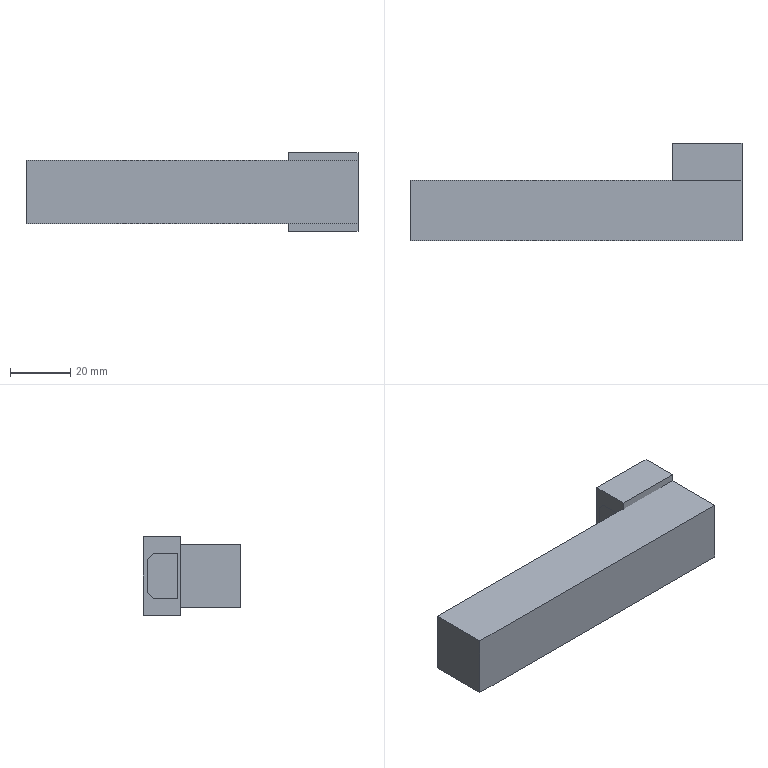CAM job | NX | 3-axis milling, drilling | part box 110 x 32.2 x 26 mm | stock box 110 x 32.2 x 26 mm
Tools:
number,name,description,diameter,corner_radius,flute_length,length,flutes
1,D16C,Milling Tool-5 Parameters,16.0,0.0,50.0,75.0,2
2,D14J,Milling Tool-5 Parameters,14.0,0.0,50.0,75.0,2
3,D4C,Milling Tool-5 Parameters,4.0,0.0,50.0,75.0,2
4,D4J,Milling Tool-5 Parameters,4.0,0.0,50.0,75.0,2
5,D4DJ,Milling Tool-5 Parameters,4.0,0.0,50.0,75.0,2
6,D8C,Milling Tool-5 Parameters,8.0,0.0,50.0,75.0,2
7,D6J,Milling Tool-5 Parameters,6.0,0.0,50.0,75.0,2
8,M6,Drilling Tool,6.0,0.0,35.0,50.0,2
Operations:
program,operation,operation_type,tool,method,geometry_group,spindle_rpm,surface_speed,feed_per_tooth,feed_cut,feed_plunge,cut_length_mm,path_length_mm,cut_time_min,machine_time_min
G54,PLANAR_MILL,PlanarMilling,D16C,METHOD,WORKPIECE,2300.0,115.0,0.1739,800.0,100.0,136.06,170.06,0.1701,0.1735
G54,ADAPTIVE_MILLING,CavityMilling,D16C,METHOD,WORKPIECE,3500.0,175.0,0.2143,1500.0,100.0,3670.104,3728.704,2.089,2.095
G54,PLANAR_MILL_1,PlanarMilling,D14J,METHOD,WORKPIECE,3000.0,131.0,0.1,600.0,100.0,569.935,695.593,0.9499,0.9625
G54,PLANAR_MILL_2,PlanarMilling,D4C,METHOD,WORKPIECE,3500.0,43.0,0.2857,2000.0,100.0,7586.181,7637.681,3.793,3.798
G54,FLOOR_WALL_1,VolumeBased25DMillingOperation,D4C,METHOD,WORKPIECE,3500.0,43.0,0.2143,1500.0,100.0,3766.549,5832.349,2.511,2.718
G54,PLANAR_MILL_2_COPY_COPY,PlanarMilling,D4DJ,METHOD,WORKPIECE,3500.0,43.0,0.1429,1000.0,100.0,150.381,188.381,0.1504,0.1542
G54,PLANAR_MILL_1_COPY,PlanarMilling,D4DJ,METHOD,WORKPIECE,3000.0,131.0,0.1,600.0,100.0,268.38,368.492,0.4473,0.4573
G54,PLANAR_MILL_2_COPY,PlanarMilling,D4J,METHOD,WORKPIECE,3500.0,43.0,0.0571,400.0,100.0,855.409,1014.041,2.139,2.154
G54,FLOOR_WALL_1_COPY,VolumeBased25DMillingOperation,D4J,METHOD,WORKPIECE,3500.0,43.0,0.0571,400.0,100.0,82.34,132.34,0.2059,0.2109
G54,PLANAR_MILL_3,PlanarMilling,D4J,METHOD,WORKPIECE,3500.0,43.0,0.0571,400.0,100.0,61.76,165.413,0.1544,0.1648
G55,PLANAR_MILL_COPY,PlanarMilling,D16C,METHOD,G55,2300.0,115.0,0.1739,800.0,100.0,136.06,170.06,0.1701,0.1735
G55,PLANAR_MILL_4,PlanarMilling,D4C,METHOD,G55,3500.0,43.0,0.1143,800.0,100.0,394.822,439.623,0.4935,0.498
G55,PLANAR_MILL_5,PlanarMilling,D4DJ,METHOD,G55,3000.0,37.0,0.1667,1000.0,100.0,174.065,269.17,0.1741,0.1836
G55,PLANAR_MILL_5_COPY,PlanarMilling,D4DJ,METHOD,G55,3000.0,37.0,0.1667,1000.0,100.0,240.912,278.912,0.2409,0.2447
G56,PLANAR_MILL_6,PlanarMilling,D16C,METHOD,WORKPIECE_1,2300.0,115.0,0.1304,600.0,100.0,53.0,87.0,0.0883,0.0917
G56,ADAPTIVE_MILLING_1,CavityMilling,D16C,METHOD,WORKPIECE_1,3500.0,175.0,0.2143,1500.0,100.0,1050.606,1122.606,0.5729,0.5801
G56,PLANAR_MILL_7,PlanarMilling,D14J,METHOD,WORKPIECE_1,3000.0,131.0,0.1,600.0,100.0,212.274,365.306,0.3538,0.3691
G56,PLANAR_MILL_7_COPY,PlanarMilling,D4DJ,METHOD,WORKPIECE_1,3000.0,131.0,0.1,600.0,100.0,119.667,196.702,0.1994,0.2071
G57,PLANAR_PROFILING,PlanarMilling,D8C,METHOD,G57,2500.0,100.0,0.0118,1000.0,100.0,2244.0,2301.0,2.244,2.25
G57,FLOOR_WALL,VolumeBased25DMillingOperation,D8C,METHOD,G57,2500.0,100.0,0.0118,1000.0,100.0,619.97,690.276,0.62,0.627
G57,FLOOR_WALL_COPY,VolumeBased25DMillingOperation,D6J,METHOD,G57,3500.0,65.0,0.0857,600.0,100.0,80.997,118.997,0.135,0.1388
G57,PLANAR_MILL_11,PlanarMilling,D6J,METHOD,G57,3500.0,65.0,0.0857,600.0,100.0,70.0,151.613,0.1167,0.1248
G57,PLANAR_MILL_8,PlanarMilling,D6J,METHOD,G57,3500.0,65.0,0.0857,600.0,100.0,31.0,87.0,0.0517,0.0573
G57,PLANAR_MILL_10,PlanarMilling,D4C,METHOD,G57,3000.0,37.0,0.1667,1000.0,100.0,502.019,554.119,0.502,0.5072
G57,PLANAR_MILL_9,PlanarMilling,D4DJ,METHOD,G57,3500.0,43.0,0.1429,1000.0,100.0,104.566,200.566,0.1046,0.1142
G57,PLANAR_MILL_9_COPY,PlanarMilling,D4DJ,METHOD,G57,3500.0,43.0,0.0857,600.0,100.0,14.254,57.854,0.0238,0.0281
G57,DRILLING,Operation,M6,METHOD,G57,300.0,5.0,0.0017,1.0,0.0,5.0,54.0,5.0,5.005